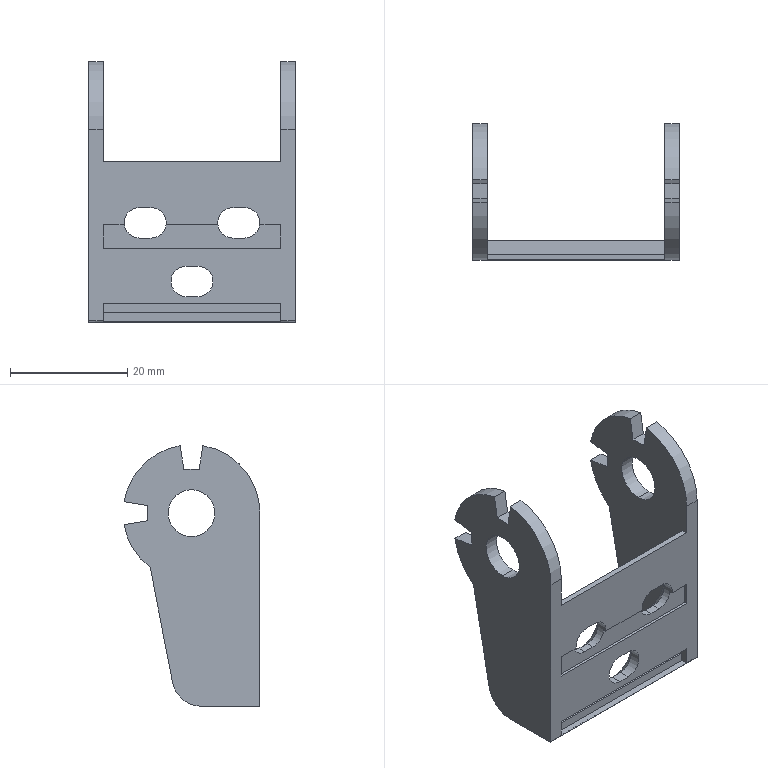Part | 1 solid | 74 faces | box 35.3 x 23.217 x 44.527 mm | volume 5659 mm3 | plane 49 | cylinder 19 | cone 6 | commonest cylinder face diameters 5.2 x6 23.38 x6 8 x4 10.1 x2 0.5 x1